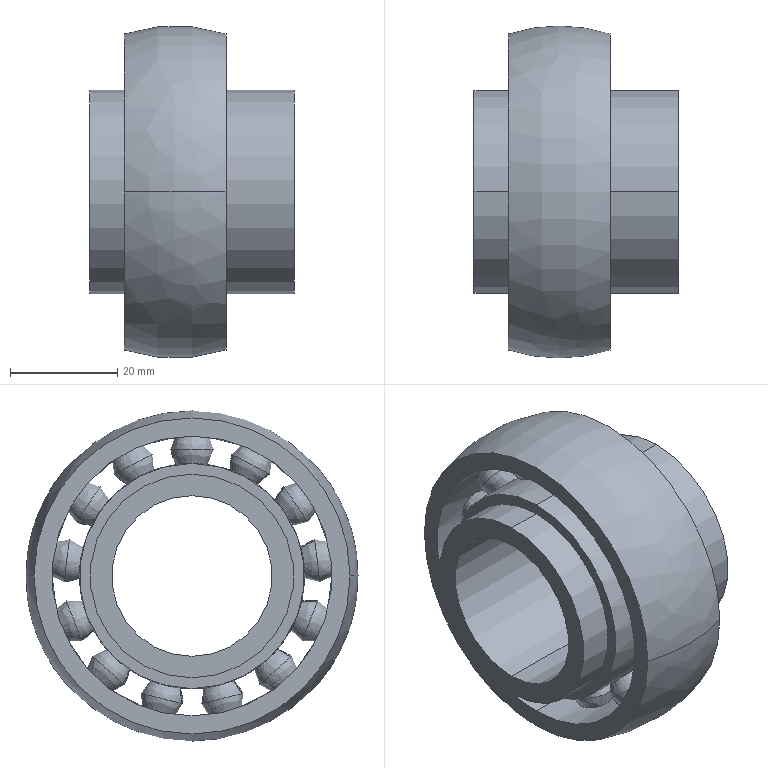Part | SolidWorks | features BaseBody 1 | 1 solid | 44 faces | box 38.1 x 62 x 62 mm | volume 38870 mm3 | spline 28 | cylinder 10 | plane 6 | commonest cylinder face diameters 38 x4 30 x2 42.044 x2 52.213 x2